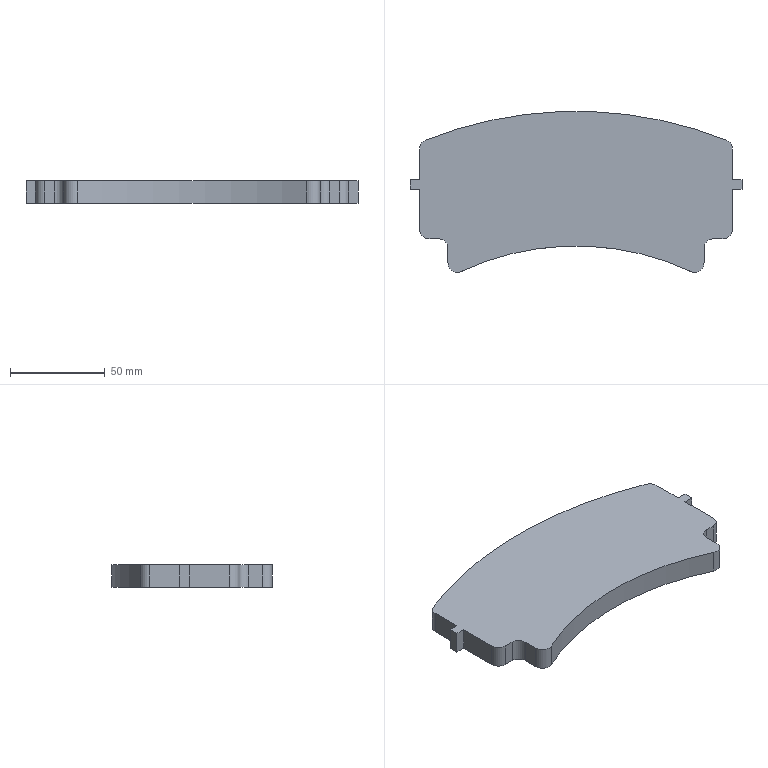Part | SolidWorks | features ICE 2, Extrusion 1, Fillet 1 | 1 solid | 26 faces | box 175 x 84.844 x 12 mm | volume 137582 mm3 | plane 16 | cylinder 10 | commonest cylinder face diameters 10 x8 286 x1 428 x1
STEP:
#1=CARTESIAN_POINT('',(-82.5,172.951,6.));
#2=VERTEX_POINT('',#1);
#3=CARTESIAN_POINT('',(-82.5,151.802,6.));
#4=VERTEX_POINT('',#3);
#5=CARTESIAN_POINT('',(-82.5,197.458,6.));
#6=DIRECTION('',(0.,-1.,0.));
#7=VECTOR('',#6,1000.);
#8=LINE('',#5,#7);
#9=EDGE_CURVE('',#2,#4,#8,.T.);
#10=ORIENTED_EDGE('',*,*,#9,.F.);
#11=CARTESIAN_POINT('',(-82.5,172.951,-6.));
#12=VERTEX_POINT('',#11);
#13=CARTESIAN_POINT('',(-82.5,172.951,-13.071));
#14=DIRECTION('',(0.,0.,1.));
#15=VECTOR('',#14,1000.);
#16=LINE('',#13,#15);
#17=EDGE_CURVE('',#12,#2,#16,.T.);
#18=ORIENTED_EDGE('',*,*,#17,.F.);
#19=CARTESIAN_POINT('',(-82.5,151.802,-6.));
#20=VERTEX_POINT('',#19);
#21=CARTESIAN_POINT('',(-82.5,197.458,-6.));
#22=DIRECTION('',(0.,-1.,0.));
#23=VECTOR('',#22,1000.);
#24=LINE('',#21,#23);
#25=EDGE_CURVE('',#12,#20,#24,.T.);
#26=ORIENTED_EDGE('',*,*,#25,.T.);
#27=CARTESIAN_POINT('',(-82.5,151.802,6.));
#28=DIRECTION('',(0.,0.,1.));
#29=VECTOR('',#28,1000.);
#30=LINE('',#27,#29);
#31=EDGE_CURVE('',#20,#4,#30,.T.);
#32=ORIENTED_EDGE('',*,*,#31,.T.);
#33=EDGE_LOOP('',(#10,#18,#26,#32));
#34=FACE_OUTER_BOUND('',#33,.T.);
#35=CARTESIAN_POINT('',(-82.5,197.458,6.));
#36=DIRECTION('',(1.,0.,0.));
#37=DIRECTION('',(0.,1.,0.));
#38=AXIS2_PLACEMENT_3D('',#35,#36,#37);
#39=PLANE('',#38);
#40=ADVANCED_FACE('',(#34),#39,.F.);
#41=CARTESIAN_POINT('',(82.5,177.951,6.));
#42=VERTEX_POINT('',#41);
#43=CARTESIAN_POINT('',(82.5,194.1,6.));
#44=VERTEX_POINT('',#43);
#45=CARTESIAN_POINT('',(82.5,197.458,6.));
#46=DIRECTION('',(0.,1.,0.));
#47=VECTOR('',#46,1000.);
#48=LINE('',#45,#47);
#49=EDGE_CURVE('',#42,#44,#48,.T.);
#50=ORIENTED_EDGE('',*,*,#49,.F.);
#51=CARTESIAN_POINT('',(82.5,177.951,-6.));
#52=VERTEX_POINT('',#51);
#53=CARTESIAN_POINT('',(82.5,177.951,-13.071));
#54=DIRECTION('',(0.,0.,1.));
#55=VECTOR('',#54,1000.);
#56=LINE('',#53,#55);
#57=EDGE_CURVE('',#52,#42,#56,.T.);
#58=ORIENTED_EDGE('',*,*,#57,.F.);
#59=CARTESIAN_POINT('',(82.5,194.1,-6.));
#60=VERTEX_POINT('',#59);
#61=CARTESIAN_POINT('',(82.5,197.458,-6.));
#62=DIRECTION('',(0.,1.,0.));
#63=VECTOR('',#62,1000.);
#64=LINE('',#61,#63);
#65=EDGE_CURVE('',#52,#60,#64,.T.);
#66=ORIENTED_EDGE('',*,*,#65,.T.);
#67=CARTESIAN_POINT('',(82.5,194.1,6.));
#68=DIRECTION('',(0.,0.,1.));
#69=VECTOR('',#68,1000.);
#70=LINE('',#67,#69);
#71=EDGE_CURVE('',#60,#44,#70,.T.);
#72=ORIENTED_EDGE('',*,*,#71,.T.);
#73=EDGE_LOOP('',(#50,#58,#66,#72));
#74=FACE_OUTER_BOUND('',#73,.T.);
#75=CARTESIAN_POINT('',(82.5,197.458,6.));
#76=DIRECTION('',(-1.,0.,0.));
#77=DIRECTION('',(0.,-1.,0.));
#78=AXIS2_PLACEMENT_3D('',#75,#76,#77);
#79=PLANE('',#78);
#80=ADVANCED_FACE('',(#74),#79,.F.);
#81=CARTESIAN_POINT('',(-60.389,129.623,-6.));
#82=VERTEX_POINT('',#81);
#83=CARTESIAN_POINT('',(60.389,129.623,-6.));
#84=VERTEX_POINT('',#83);
#85=CARTESIAN_POINT('',(0.,0.,-6.));
#86=DIRECTION('',(0.,0.,-1.));
#87=DIRECTION('',(1.,0.,0.));
#88=AXIS2_PLACEMENT_3D('',#85,#86,#87);
#89=CIRCLE('',#88,143.);
#90=EDGE_CURVE('',#82,#84,#89,.T.);
#91=ORIENTED_EDGE('',*,*,#90,.T.);
#92=CARTESIAN_POINT('',(60.389,129.623,6.));
#93=VERTEX_POINT('',#92);
#94=CARTESIAN_POINT('',(60.389,129.623,6.));
#95=DIRECTION('',(0.,0.,1.));
#96=VECTOR('',#95,1000.);
#97=LINE('',#94,#96);
#98=EDGE_CURVE('',#84,#93,#97,.T.);
#99=ORIENTED_EDGE('',*,*,#98,.T.);
#100=CARTESIAN_POINT('',(-60.389,129.623,6.));
#101=VERTEX_POINT('',#100);
#102=CARTESIAN_POINT('',(0.,0.,6.));
#103=DIRECTION('',(0.,0.,-1.));
#104=DIRECTION('',(1.,0.,0.));
#105=AXIS2_PLACEMENT_3D('',#102,#103,#104);
#106=CIRCLE('',#105,143.);
#107=EDGE_CURVE('',#101,#93,#106,.T.);
#108=ORIENTED_EDGE('',*,*,#107,.F.);
#109=CARTESIAN_POINT('',(-60.389,129.623,6.));
#110=DIRECTION('',(0.,0.,-1.));
#111=VECTOR('',#110,1000.);
#112=LINE('',#109,#111);
#113=EDGE_CURVE('',#101,#82,#112,.T.);
#114=ORIENTED_EDGE('',*,*,#113,.T.);
#115=EDGE_LOOP('',(#91,#99,#108,#114));
#116=FACE_OUTER_BOUND('',#115,.T.);
#117=CARTESIAN_POINT('',(0.,0.,6.));
#118=DIRECTION('',(0.,0.,-1.));
#119=DIRECTION('',(-1.,0.,0.));
#120=AXIS2_PLACEMENT_3D('',#117,#118,#119);
#121=CYLINDRICAL_SURFACE('',#120,143.);
#122=ADVANCED_FACE('',(#116),#121,.F.);
#123=CARTESIAN_POINT('',(82.5,151.802,-6.));
#124=VERTEX_POINT('',#123);
#125=CARTESIAN_POINT('',(82.5,172.951,-6.));
#126=VERTEX_POINT('',#125);
#127=CARTESIAN_POINT('',(82.5,197.458,-6.));
#128=DIRECTION('',(0.,1.,0.));
#129=VECTOR('',#128,1000.);
#130=LINE('',#127,#129);
#131=EDGE_CURVE('',#124,#126,#130,.T.);
#132=ORIENTED_EDGE('',*,*,#131,.T.);
#133=CARTESIAN_POINT('',(82.5,172.951,6.));
#134=VERTEX_POINT('',#133);
#135=CARTESIAN_POINT('',(82.5,172.951,-13.071));
#136=DIRECTION('',(0.,0.,1.));
#137=VECTOR('',#136,1000.);
#138=LINE('',#135,#137);
#139=EDGE_CURVE('',#126,#134,#138,.T.);
#140=ORIENTED_EDGE('',*,*,#139,.T.);
#141=CARTESIAN_POINT('',(82.5,151.802,6.));
#142=VERTEX_POINT('',#141);
#143=CARTESIAN_POINT('',(82.5,197.458,6.));
#144=DIRECTION('',(0.,1.,0.));
#145=VECTOR('',#144,1000.);
#146=LINE('',#143,#145);
#147=EDGE_CURVE('',#142,#134,#146,.T.);
#148=ORIENTED_EDGE('',*,*,#147,.F.);
#149=CARTESIAN_POINT('',(82.5,151.802,6.));
#150=DIRECTION('',(0.,0.,-1.));
#151=VECTOR('',#150,1000.);
#152=LINE('',#149,#151);
#153=EDGE_CURVE('',#142,#124,#152,.T.);
#154=ORIENTED_EDGE('',*,*,#153,.T.);
#155=EDGE_LOOP('',(#132,#140,#148,#154));
#156=FACE_OUTER_BOUND('',#155,.T.);
#157=CARTESIAN_POINT('',(82.5,197.458,6.));
#158=DIRECTION('',(-1.,0.,0.));
#159=DIRECTION('',(0.,-1.,0.));
#160=AXIS2_PLACEMENT_3D('',#157,#158,#159);
#161=PLANE('',#160);
#162=ADVANCED_FACE('',(#156),#161,.F.);
#163=CARTESIAN_POINT('',(79.354,198.743,6.));
#164=VERTEX_POINT('',#163);
#165=CARTESIAN_POINT('',(-79.354,198.743,6.));
#166=VERTEX_POINT('',#165);
#167=CARTESIAN_POINT('',(0.,0.,6.));
#168=DIRECTION('',(0.,0.,1.));
#169=DIRECTION('',(1.,0.,0.));
#170=AXIS2_PLACEMENT_3D('',#167,#168,#169);
#171=CIRCLE('',#170,214.);
#172=EDGE_CURVE('',#164,#166,#171,.T.);
#173=ORIENTED_EDGE('',*,*,#172,.F.);
#174=CARTESIAN_POINT('',(79.354,198.743,-6.));
#175=VERTEX_POINT('',#174);
#176=CARTESIAN_POINT('',(79.354,198.743,6.));
#177=DIRECTION('',(0.,0.,-1.));
#178=VECTOR('',#177,1000.);
#179=LINE('',#176,#178);
#180=EDGE_CURVE('',#164,#175,#179,.T.);
#181=ORIENTED_EDGE('',*,*,#180,.T.);
#182=CARTESIAN_POINT('',(-79.354,198.743,-6.));
#183=VERTEX_POINT('',#182);
#184=CARTESIAN_POINT('',(0.,0.,-6.));
#185=DIRECTION('',(0.,0.,1.));
#186=DIRECTION('',(1.,0.,0.));
#187=AXIS2_PLACEMENT_3D('',#184,#185,#186);
#188=CIRCLE('',#187,214.);
#189=EDGE_CURVE('',#175,#183,#188,.T.);
#190=ORIENTED_EDGE('',*,*,#189,.T.);
#191=CARTESIAN_POINT('',(-79.354,198.743,6.));
#192=DIRECTION('',(0.,0.,1.));
#193=VECTOR('',#192,1000.);
#194=LINE('',#191,#193);
#195=EDGE_CURVE('',#183,#166,#194,.T.);
#196=ORIENTED_EDGE('',*,*,#195,.T.);
#197=EDGE_LOOP('',(#173,#181,#190,#196));
#198=FACE_OUTER_BOUND('',#197,.T.);
#199=CARTESIAN_POINT('',(0.,0.,6.));
#200=DIRECTION('',(0.,0.,-1.));
#201=DIRECTION('',(-1.,0.,0.));
#202=AXIS2_PLACEMENT_3D('',#199,#200,#201);
#203=CYLINDRICAL_SURFACE('',#202,214.);
#204=ADVANCED_FACE('',(#198),#203,.T.);
#205=CARTESIAN_POINT('',(-82.5,194.1,-6.));
#206=VERTEX_POINT('',#205);
#207=CARTESIAN_POINT('',(-82.5,177.951,-6.));
#208=VERTEX_POINT('',#207);
#209=CARTESIAN_POINT('',(-82.5,197.458,-6.));
#210=DIRECTION('',(0.,-1.,0.));
#211=VECTOR('',#210,1000.);
#212=LINE('',#209,#211);
#213=EDGE_CURVE('',#206,#208,#212,.T.);
#214=ORIENTED_EDGE('',*,*,#213,.T.);
#215=CARTESIAN_POINT('',(-82.5,177.951,6.));
#216=VERTEX_POINT('',#215);
#217=CARTESIAN_POINT('',(-82.5,177.951,-13.071));
#218=DIRECTION('',(0.,0.,1.));
#219=VECTOR('',#218,1000.);
#220=LINE('',#217,#219);
#221=EDGE_CURVE('',#208,#216,#220,.T.);
#222=ORIENTED_EDGE('',*,*,#221,.T.);
#223=CARTESIAN_POINT('',(-82.5,194.1,6.));
#224=VERTEX_POINT('',#223);
#225=CARTESIAN_POINT('',(-82.5,197.458,6.));
#226=DIRECTION('',(0.,-1.,0.));
#227=VECTOR('',#226,1000.);
#228=LINE('',#225,#227);
#229=EDGE_CURVE('',#224,#216,#228,.T.);
#230=ORIENTED_EDGE('',*,*,#229,.F.);
#231=CARTESIAN_POINT('',(-82.5,194.1,6.));
#232=DIRECTION('',(0.,0.,-1.));
#233=VECTOR('',#232,1000.);
#234=LINE('',#231,#233);
#235=EDGE_CURVE('',#224,#206,#234,.T.);
#236=ORIENTED_EDGE('',*,*,#235,.T.);
#237=EDGE_LOOP('',(#214,#222,#230,#236));
#238=FACE_OUTER_BOUND('',#237,.T.);
#239=CARTESIAN_POINT('',(-82.5,197.458,6.));
#240=DIRECTION('',(1.,0.,0.));
#241=DIRECTION('',(0.,1.,0.));
#242=AXIS2_PLACEMENT_3D('',#239,#240,#241);
#243=PLANE('',#242);
#244=ADVANCED_FACE('',(#238),#243,.F.);
#245=ORIENTED_EDGE('',*,*,#147,.T.);
#246=CARTESIAN_POINT('',(87.5,172.951,6.));
#247=VERTEX_POINT('',#246);
#248=CARTESIAN_POINT('',(82.5,172.951,6.));
#249=DIRECTION('',(1.,0.,0.));
#250=VECTOR('',#249,1000.);
#251=LINE('',#248,#250);
#252=EDGE_CURVE('',#134,#247,#251,.T.);
#253=ORIENTED_EDGE('',*,*,#252,.T.);
#254=CARTESIAN_POINT('',(87.5,177.951,6.));
#255=VERTEX_POINT('',#254);
#256=CARTESIAN_POINT('',(87.5,172.951,6.));
#257=DIRECTION('',(0.,1.,0.));
#258=VECTOR('',#257,1000.);
#259=LINE('',#256,#258);
#260=EDGE_CURVE('',#247,#255,#259,.T.);
#261=ORIENTED_EDGE('',*,*,#260,.T.);
#262=CARTESIAN_POINT('',(82.5,177.951,6.));
#263=DIRECTION('',(-1.,0.,0.));
#264=VECTOR('',#263,1000.);
#265=LINE('',#262,#264);
#266=EDGE_CURVE('',#255,#42,#265,.T.);
#267=ORIENTED_EDGE('',*,*,#266,.T.);
#268=ORIENTED_EDGE('',*,*,#49,.T.);
#269=CARTESIAN_POINT('',(77.5,194.1,6.));
#270=DIRECTION('',(0.,0.,1.));
#271=DIRECTION('',(1.,0.,0.));
#272=AXIS2_PLACEMENT_3D('',#269,#270,#271);
#273=CIRCLE('',#272,5.);
#274=EDGE_CURVE('',#44,#164,#273,.T.);
#275=ORIENTED_EDGE('',*,*,#274,.T.);
#276=ORIENTED_EDGE('',*,*,#172,.T.);
#277=CARTESIAN_POINT('',(-77.5,194.1,6.));
#278=DIRECTION('',(0.,0.,1.));
#279=DIRECTION('',(1.,0.,0.));
#280=AXIS2_PLACEMENT_3D('',#277,#278,#279);
#281=CIRCLE('',#280,5.);
#282=EDGE_CURVE('',#166,#224,#281,.T.);
#283=ORIENTED_EDGE('',*,*,#282,.T.);
#284=ORIENTED_EDGE('',*,*,#229,.T.);
#285=CARTESIAN_POINT('',(-87.5,177.951,6.));
#286=VERTEX_POINT('',#285);
#287=CARTESIAN_POINT('',(-82.5,177.951,6.));
#288=DIRECTION('',(-1.,0.,0.));
#289=VECTOR('',#288,1000.);
#290=LINE('',#287,#289);
#291=EDGE_CURVE('',#216,#286,#290,.T.);
#292=ORIENTED_EDGE('',*,*,#291,.T.);
#293=CARTESIAN_POINT('',(-87.5,172.951,6.));
#294=VERTEX_POINT('',#293);
#295=CARTESIAN_POINT('',(-87.5,172.951,6.));
#296=DIRECTION('',(0.,-1.,0.));
#297=VECTOR('',#296,1000.);
#298=LINE('',#295,#297);
#299=EDGE_CURVE('',#286,#294,#298,.T.);
#300=ORIENTED_EDGE('',*,*,#299,.T.);
#301=CARTESIAN_POINT('',(-82.5,172.951,6.));
#302=DIRECTION('',(1.,0.,0.));
#303=VECTOR('',#302,1000.);
#304=LINE('',#301,#303);
#305=EDGE_CURVE('',#294,#2,#304,.T.);
#306=ORIENTED_EDGE('',*,*,#305,.T.);
#307=ORIENTED_EDGE('',*,*,#9,.T.);
#308=CARTESIAN_POINT('',(-77.5,146.802,6.));
#309=VERTEX_POINT('',#308);
#310=CARTESIAN_POINT('',(-77.5,151.802,6.));
#311=DIRECTION('',(0.,0.,1.));
#312=DIRECTION('',(1.,0.,0.));
#313=AXIS2_PLACEMENT_3D('',#310,#311,#312);
#314=CIRCLE('',#313,5.);
#315=EDGE_CURVE('',#4,#309,#314,.T.);
#316=ORIENTED_EDGE('',*,*,#315,.T.);
#317=CARTESIAN_POINT('',(-72.5,146.802,6.));
#318=VERTEX_POINT('',#317);
#319=CARTESIAN_POINT('',(-82.5,146.802,6.));
#320=DIRECTION('',(-1.,0.,0.));
#321=VECTOR('',#320,1000.);
#322=LINE('',#319,#321);
#323=EDGE_CURVE('',#318,#309,#322,.T.);
#324=ORIENTED_EDGE('',*,*,#323,.F.);
#325=CARTESIAN_POINT('',(-67.5,141.802,6.));
#326=VERTEX_POINT('',#325);
#327=CARTESIAN_POINT('',(-72.5,141.802,6.));
#328=DIRECTION('',(0.,0.,-1.));
#329=DIRECTION('',(1.,0.,0.));
#330=AXIS2_PLACEMENT_3D('',#327,#328,#329);
#331=CIRCLE('',#330,5.);
#332=EDGE_CURVE('',#318,#326,#331,.T.);
#333=ORIENTED_EDGE('',*,*,#332,.T.);
#334=CARTESIAN_POINT('',(-67.5,134.156,6.));
#335=VERTEX_POINT('',#334);
#336=CARTESIAN_POINT('',(-67.5,116.802,6.));
#337=DIRECTION('',(0.,1.,0.));
#338=VECTOR('',#337,1000.);
#339=LINE('',#336,#338);
#340=EDGE_CURVE('',#335,#326,#339,.T.);
#341=ORIENTED_EDGE('',*,*,#340,.F.);
#342=CARTESIAN_POINT('',(-62.5,134.156,6.));
#343=DIRECTION('',(0.,0.,1.));
#344=DIRECTION('',(1.,0.,0.));
#345=AXIS2_PLACEMENT_3D('',#342,#343,#344);
#346=CIRCLE('',#345,5.);
#347=EDGE_CURVE('',#335,#101,#346,.T.);
#348=ORIENTED_EDGE('',*,*,#347,.T.);
#349=ORIENTED_EDGE('',*,*,#107,.T.);
#350=CARTESIAN_POINT('',(67.5,134.156,6.));
#351=VERTEX_POINT('',#350);
#352=CARTESIAN_POINT('',(62.5,134.156,6.));
#353=DIRECTION('',(0.,0.,1.));
#354=DIRECTION('',(1.,0.,0.));
#355=AXIS2_PLACEMENT_3D('',#352,#353,#354);
#356=CIRCLE('',#355,5.);
#357=EDGE_CURVE('',#93,#351,#356,.T.);
#358=ORIENTED_EDGE('',*,*,#357,.T.);
#359=CARTESIAN_POINT('',(67.5,141.802,6.));
#360=VERTEX_POINT('',#359);
#361=CARTESIAN_POINT('',(67.5,116.802,6.));
#362=DIRECTION('',(0.,-1.,0.));
#363=VECTOR('',#362,1000.);
#364=LINE('',#361,#363);
#365=EDGE_CURVE('',#360,#351,#364,.T.);
#366=ORIENTED_EDGE('',*,*,#365,.F.);
#367=CARTESIAN_POINT('',(72.5,146.802,6.));
#368=VERTEX_POINT('',#367);
#369=CARTESIAN_POINT('',(72.5,141.802,6.));
#370=DIRECTION('',(0.,0.,-1.));
#371=DIRECTION('',(1.,0.,0.));
#372=AXIS2_PLACEMENT_3D('',#369,#370,#371);
#373=CIRCLE('',#372,5.);
#374=EDGE_CURVE('',#360,#368,#373,.T.);
#375=ORIENTED_EDGE('',*,*,#374,.T.);
#376=CARTESIAN_POINT('',(77.5,146.802,6.));
#377=VERTEX_POINT('',#376);
#378=CARTESIAN_POINT('',(82.5,146.802,6.));
#379=DIRECTION('',(-1.,0.,0.));
#380=VECTOR('',#379,1000.);
#381=LINE('',#378,#380);
#382=EDGE_CURVE('',#377,#368,#381,.T.);
#383=ORIENTED_EDGE('',*,*,#382,.F.);
#384=CARTESIAN_POINT('',(77.5,151.802,6.));
#385=DIRECTION('',(0.,0.,1.));
#386=DIRECTION('',(1.,0.,0.));
#387=AXIS2_PLACEMENT_3D('',#384,#385,#386);
#388=CIRCLE('',#387,5.);
#389=EDGE_CURVE('',#377,#142,#388,.T.);
#390=ORIENTED_EDGE('',*,*,#389,.T.);
#391=EDGE_LOOP('',(#245,#253,#261,#267,#268,#275,#276,#283,#284,#292,#300,#306,#307,#316,#324,#333,#341,#348,#349,#358,#366,#375,#383,#390));
#392=FACE_OUTER_BOUND('',#391,.T.);
#393=CARTESIAN_POINT('',(0.,0.,6.));
#394=DIRECTION('',(0.,0.,1.));
#395=DIRECTION('',(1.,0.,0.));
#396=AXIS2_PLACEMENT_3D('',#393,#394,#395);
#397=PLANE('',#396);
#398=ADVANCED_FACE('',(#392),#397,.T.);
#399=ORIENTED_EDGE('',*,*,#189,.F.);
#400=CARTESIAN_POINT('',(77.5,194.1,-6.));
#401=DIRECTION('',(0.,0.,-1.));
#402=DIRECTION('',(1.,0.,0.));
#403=AXIS2_PLACEMENT_3D('',#400,#401,#402);
#404=CIRCLE('',#403,5.);
#405=EDGE_CURVE('',#175,#60,#404,.T.);
#406=ORIENTED_EDGE('',*,*,#405,.T.);
#407=ORIENTED_EDGE('',*,*,#65,.F.);
#408=CARTESIAN_POINT('',(87.5,177.951,-6.));
#409=VERTEX_POINT('',#408);
#410=CARTESIAN_POINT('',(82.5,177.951,-6.));
#411=DIRECTION('',(1.,0.,0.));
#412=VECTOR('',#411,1000.);
#413=LINE('',#410,#412);
#414=EDGE_CURVE('',#52,#409,#413,.T.);
#415=ORIENTED_EDGE('',*,*,#414,.T.);
#416=CARTESIAN_POINT('',(87.5,172.951,-6.));
#417=VERTEX_POINT('',#416);
#418=CARTESIAN_POINT('',(87.5,172.951,-6.));
#419=DIRECTION('',(0.,-1.,0.));
#420=VECTOR('',#419,1000.);
#421=LINE('',#418,#420);
#422=EDGE_CURVE('',#409,#417,#421,.T.);
#423=ORIENTED_EDGE('',*,*,#422,.T.);
#424=CARTESIAN_POINT('',(82.5,172.951,-6.));
#425=DIRECTION('',(-1.,0.,0.));
#426=VECTOR('',#425,1000.);
#427=LINE('',#424,#426);
#428=EDGE_CURVE('',#417,#126,#427,.T.);
#429=ORIENTED_EDGE('',*,*,#428,.T.);
#430=ORIENTED_EDGE('',*,*,#131,.F.);
#431=CARTESIAN_POINT('',(77.5,146.802,-6.));
#432=VERTEX_POINT('',#431);
#433=CARTESIAN_POINT('',(77.5,151.802,-6.));
#434=DIRECTION('',(0.,0.,-1.));
#435=DIRECTION('',(1.,0.,0.));
#436=AXIS2_PLACEMENT_3D('',#433,#434,#435);
#437=CIRCLE('',#436,5.);
#438=EDGE_CURVE('',#124,#432,#437,.T.);
#439=ORIENTED_EDGE('',*,*,#438,.T.);
#440=CARTESIAN_POINT('',(72.5,146.802,-6.));
#441=VERTEX_POINT('',#440);
#442=CARTESIAN_POINT('',(0.,146.802,-6.));
#443=DIRECTION('',(-1.,0.,0.));
#444=VECTOR('',#443,1000.);
#445=LINE('',#442,#444);
#446=EDGE_CURVE('',#432,#441,#445,.T.);
#447=ORIENTED_EDGE('',*,*,#446,.T.);
#448=CARTESIAN_POINT('',(67.5,141.802,-6.));
#449=VERTEX_POINT('',#448);
#450=CARTESIAN_POINT('',(72.5,141.802,-6.));
#451=DIRECTION('',(0.,0.,1.));
#452=DIRECTION('',(1.,0.,0.));
#453=AXIS2_PLACEMENT_3D('',#450,#451,#452);
#454=CIRCLE('',#453,5.);
#455=EDGE_CURVE('',#441,#449,#454,.T.);
#456=ORIENTED_EDGE('',*,*,#455,.T.);
#457=CARTESIAN_POINT('',(67.5,134.156,-6.));
#458=VERTEX_POINT('',#457);
#459=CARTESIAN_POINT('',(67.5,0.,-6.));
#460=DIRECTION('',(0.,-1.,0.));
#461=VECTOR('',#460,1000.);
#462=LINE('',#459,#461);
#463=EDGE_CURVE('',#449,#458,#462,.T.);
#464=ORIENTED_EDGE('',*,*,#463,.T.);
#465=CARTESIAN_POINT('',(62.5,134.156,-6.));
#466=DIRECTION('',(0.,0.,-1.));
#467=DIRECTION('',(1.,0.,0.));
#468=AXIS2_PLACEMENT_3D('',#465,#466,#467);
#469=CIRCLE('',#468,5.);
#470=EDGE_CURVE('',#458,#84,#469,.T.);
#471=ORIENTED_EDGE('',*,*,#470,.T.);
#472=ORIENTED_EDGE('',*,*,#90,.F.);
#473=CARTESIAN_POINT('',(-67.5,134.156,-6.));
#474=VERTEX_POINT('',#473);
#475=CARTESIAN_POINT('',(-62.5,134.156,-6.));
#476=DIRECTION('',(0.,0.,-1.));
#477=DIRECTION('',(1.,0.,0.));
#478=AXIS2_PLACEMENT_3D('',#475,#476,#477);
#479=CIRCLE('',#478,5.);
#480=EDGE_CURVE('',#82,#474,#479,.T.);
#481=ORIENTED_EDGE('',*,*,#480,.T.);
#482=CARTESIAN_POINT('',(-67.5,141.802,-6.));
#483=VERTEX_POINT('',#482);
#484=CARTESIAN_POINT('',(-67.5,0.,-6.));
#485=DIRECTION('',(0.,1.,0.));
#486=VECTOR('',#485,1000.);
#487=LINE('',#484,#486);
#488=EDGE_CURVE('',#474,#483,#487,.T.);
#489=ORIENTED_EDGE('',*,*,#488,.T.);
#490=CARTESIAN_POINT('',(-72.5,146.802,-6.));
#491=VERTEX_POINT('',#490);
#492=CARTESIAN_POINT('',(-72.5,141.802,-6.));
#493=DIRECTION('',(0.,0.,1.));
#494=DIRECTION('',(1.,0.,0.));
#495=AXIS2_PLACEMENT_3D('',#492,#493,#494);
#496=CIRCLE('',#495,5.);
#497=EDGE_CURVE('',#483,#491,#496,.T.);
#498=ORIENTED_EDGE('',*,*,#497,.T.);
#499=CARTESIAN_POINT('',(-77.5,146.802,-6.));
#500=VERTEX_POINT('',#499);
#501=CARTESIAN_POINT('',(0.,146.802,-6.));
#502=DIRECTION('',(-1.,0.,0.));
#503=VECTOR('',#502,1000.);
#504=LINE('',#501,#503);
#505=EDGE_CURVE('',#491,#500,#504,.T.);
#506=ORIENTED_EDGE('',*,*,#505,.T.);
#507=CARTESIAN_POINT('',(-77.5,151.802,-6.));
#508=DIRECTION('',(0.,0.,-1.));
#509=DIRECTION('',(1.,0.,0.));
#510=AXIS2_PLACEMENT_3D('',#507,#508,#509);
#511=CIRCLE('',#510,5.);
#512=EDGE_CURVE('',#500,#20,#511,.T.);
#513=ORIENTED_EDGE('',*,*,#512,.T.);
#514=ORIENTED_EDGE('',*,*,#25,.F.);
#515=CARTESIAN_POINT('',(-87.5,172.951,-6.));
#516=VERTEX_POINT('',#515);
#517=CARTESIAN_POINT('',(-82.5,172.951,-6.));
#518=DIRECTION('',(-1.,0.,0.));
#519=VECTOR('',#518,1000.);
#520=LINE('',#517,#519);
#521=EDGE_CURVE('',#12,#516,#520,.T.);
#522=ORIENTED_EDGE('',*,*,#521,.T.);
#523=CARTESIAN_POINT('',(-87.5,177.951,-6.));
#524=VERTEX_POINT('',#523);
#525=CARTESIAN_POINT('',(-87.5,172.951,-6.));
#526=DIRECTION('',(0.,1.,0.));
#527=VECTOR('',#526,1000.);
#528=LINE('',#525,#527);
#529=EDGE_CURVE('',#516,#524,#528,.T.);
#530=ORIENTED_EDGE('',*,*,#529,.T.);
#531=CARTESIAN_POINT('',(-82.5,177.951,-6.));
#532=DIRECTION('',(1.,0.,0.));
#533=VECTOR('',#532,1000.);
#534=LINE('',#531,#533);
#535=EDGE_CURVE('',#524,#208,#534,.T.);
#536=ORIENTED_EDGE('',*,*,#535,.T.);
#537=ORIENTED_EDGE('',*,*,#213,.F.);
#538=CARTESIAN_POINT('',(-77.5,194.1,-6.));
#539=DIRECTION('',(0.,0.,-1.));
#540=DIRECTION('',(1.,0.,0.));
#541=AXIS2_PLACEMENT_3D('',#538,#539,#540);
#542=CIRCLE('',#541,5.);
#543=EDGE_CURVE('',#206,#183,#542,.T.);
#544=ORIENTED_EDGE('',*,*,#543,.T.);
#545=EDGE_LOOP('',(#399,#406,#407,#415,#423,#429,#430,#439,#447,#456,#464,#471,#472,#481,#489,#498,#506,#513,#514,#522,#530,#536,#537,#544));
#546=FACE_OUTER_BOUND('',#545,.T.);
#547=CARTESIAN_POINT('',(0.,0.,-6.));
#548=DIRECTION('',(0.,0.,1.));
#549=DIRECTION('',(1.,0.,0.));
#550=AXIS2_PLACEMENT_3D('',#547,#548,#549);
#551=PLANE('',#550);
#552=ADVANCED_FACE('',(#546),#551,.F.);
#553=ORIENTED_EDGE('',*,*,#463,.F.);
#554=CARTESIAN_POINT('',(67.5,141.802,6.));
#555=DIRECTION('',(0.,0.,1.));
#556=VECTOR('',#555,1000.);
#557=LINE('',#554,#556);
#558=EDGE_CURVE('',#449,#360,#557,.T.);
#559=ORIENTED_EDGE('',*,*,#558,.T.);
#560=ORIENTED_EDGE('',*,*,#365,.T.);
#561=CARTESIAN_POINT('',(67.5,134.156,-24.));
#562=DIRECTION('',(0.,0.,-1.));
#563=VECTOR('',#562,1000.);
#564=LINE('',#561,#563);
#565=EDGE_CURVE('',#351,#458,#564,.T.);
#566=ORIENTED_EDGE('',*,*,#565,.T.);
#567=EDGE_LOOP('',(#553,#559,#560,#566));
#568=FACE_OUTER_BOUND('',#567,.T.);
#569=CARTESIAN_POINT('',(67.5,116.802,-24.));
#570=DIRECTION('',(-1.,0.,0.));
#571=DIRECTION('',(0.,0.,1.));
#572=AXIS2_PLACEMENT_3D('',#569,#570,#571);
#573=PLANE('',#572);
#574=ADVANCED_FACE('',(#568),#573,.F.);
#575=ORIENTED_EDGE('',*,*,#446,.F.);
#576=CARTESIAN_POINT('',(77.5,146.802,-24.));
#577=DIRECTION('',(0.,0.,1.));
#578=VECTOR('',#577,1000.);
#579=LINE('',#576,#578);
#580=EDGE_CURVE('',#432,#377,#579,.T.);
#581=ORIENTED_EDGE('',*,*,#580,.T.);
#582=ORIENTED_EDGE('',*,*,#382,.T.);
#583=CARTESIAN_POINT('',(72.5,146.802,-6.));
#584=DIRECTION('',(0.,0.,-1.));
#585=VECTOR('',#584,1000.);
#586=LINE('',#583,#585);
#587=EDGE_CURVE('',#368,#441,#586,.T.);
#588=ORIENTED_EDGE('',*,*,#587,.T.);
#589=EDGE_LOOP('',(#575,#581,#582,#588));
#590=FACE_OUTER_BOUND('',#589,.T.);
#591=CARTESIAN_POINT('',(82.5,146.802,-24.));
#592=DIRECTION('',(0.,1.,0.));
#593=DIRECTION('',(0.,0.,1.));
#594=AXIS2_PLACEMENT_3D('',#591,#592,#593);
#595=PLANE('',#594);
#596=ADVANCED_FACE('',(#590),#595,.F.);
#597=ORIENTED_EDGE('',*,*,#505,.F.);
#598=CARTESIAN_POINT('',(-72.5,146.802,6.));
#599=DIRECTION('',(0.,0.,1.));
#600=VECTOR('',#599,1000.);
#601=LINE('',#598,#600);
#602=EDGE_CURVE('',#491,#318,#601,.T.);
#603=ORIENTED_EDGE('',*,*,#602,.T.);
#604=ORIENTED_EDGE('',*,*,#323,.T.);
#605=CARTESIAN_POINT('',(-77.5,146.802,-24.));
#606=DIRECTION('',(0.,0.,-1.));
#607=VECTOR('',#606,1000.);
#608=LINE('',#605,#607);
#609=EDGE_CURVE('',#309,#500,#608,.T.);
#610=ORIENTED_EDGE('',*,*,#609,.T.);
#611=EDGE_LOOP('',(#597,#603,#604,#610));
#612=FACE_OUTER_BOUND('',#611,.T.);
#613=CARTESIAN_POINT('',(-82.5,146.802,-24.));
#614=DIRECTION('',(0.,1.,0.));
#615=DIRECTION('',(0.,0.,1.));
#616=AXIS2_PLACEMENT_3D('',#613,#614,#615);
#617=PLANE('',#616);
#618=ADVANCED_FACE('',(#612),#617,.F.);
#619=ORIENTED_EDGE('',*,*,#488,.F.);
#620=CARTESIAN_POINT('',(-67.5,134.156,-24.));
#621=DIRECTION('',(0.,0.,1.));
#622=VECTOR('',#621,1000.);
#623=LINE('',#620,#622);
#624=EDGE_CURVE('',#474,#335,#623,.T.);
#625=ORIENTED_EDGE('',*,*,#624,.T.);
#626=ORIENTED_EDGE('',*,*,#340,.T.);
#627=CARTESIAN_POINT('',(-67.5,141.802,-6.));
#628=DIRECTION('',(0.,0.,-1.));
#629=VECTOR('',#628,1000.);
#630=LINE('',#627,#629);
#631=EDGE_CURVE('',#326,#483,#630,.T.);
#632=ORIENTED_EDGE('',*,*,#631,.T.);
#633=EDGE_LOOP('',(#619,#625,#626,#632));
#634=FACE_OUTER_BOUND('',#633,.T.);
#635=CARTESIAN_POINT('',(-67.5,116.802,-24.));
#636=DIRECTION('',(1.,0.,0.));
#637=DIRECTION('',(0.,0.,-1.));
#638=AXIS2_PLACEMENT_3D('',#635,#636,#637);
#639=PLANE('',#638);
#640=ADVANCED_FACE('',(#634),#639,.F.);
#641=ORIENTED_EDGE('',*,*,#274,.F.);
#642=ORIENTED_EDGE('',*,*,#71,.F.);
#643=ORIENTED_EDGE('',*,*,#405,.F.);
#644=ORIENTED_EDGE('',*,*,#180,.F.);
#645=EDGE_LOOP('',(#641,#642,#643,#644));
#646=FACE_OUTER_BOUND('',#645,.T.);
#647=CARTESIAN_POINT('',(77.5,194.1,6.));
#648=DIRECTION('',(0.,0.,-1.));
#649=DIRECTION('',(-1.,0.,0.));
#650=AXIS2_PLACEMENT_3D('',#647,#648,#649);
#651=CYLINDRICAL_SURFACE('',#650,5.);
#652=ADVANCED_FACE('',(#646),#651,.T.);
#653=ORIENTED_EDGE('',*,*,#438,.F.);
#654=ORIENTED_EDGE('',*,*,#153,.F.);
#655=ORIENTED_EDGE('',*,*,#389,.F.);
#656=ORIENTED_EDGE('',*,*,#580,.F.);
#657=EDGE_LOOP('',(#653,#654,#655,#656));
#658=FACE_OUTER_BOUND('',#657,.T.);
#659=CARTESIAN_POINT('',(77.5,151.802,-24.));
#660=DIRECTION('',(0.,0.,1.));
#661=DIRECTION('',(1.,0.,0.));
#662=AXIS2_PLACEMENT_3D('',#659,#660,#661);
#663=CYLINDRICAL_SURFACE('',#662,5.);
#664=ADVANCED_FACE('',(#658),#663,.T.);
#665=ORIENTED_EDGE('',*,*,#455,.F.);
#666=ORIENTED_EDGE('',*,*,#587,.F.);
#667=ORIENTED_EDGE('',*,*,#374,.F.);
#668=ORIENTED_EDGE('',*,*,#558,.F.);
#669=EDGE_LOOP('',(#665,#666,#667,#668));
#670=FACE_OUTER_BOUND('',#669,.T.);
#671=CARTESIAN_POINT('',(72.5,141.802,-24.));
#672=DIRECTION('',(0.,0.,-1.));
#673=DIRECTION('',(-1.,0.,0.));
#674=AXIS2_PLACEMENT_3D('',#671,#672,#673);
#675=CYLINDRICAL_SURFACE('',#674,5.);
#676=ADVANCED_FACE('',(#670),#675,.F.);
#677=ORIENTED_EDGE('',*,*,#470,.F.);
#678=ORIENTED_EDGE('',*,*,#565,.F.);
#679=ORIENTED_EDGE('',*,*,#357,.F.);
#680=ORIENTED_EDGE('',*,*,#98,.F.);
#681=EDGE_LOOP('',(#677,#678,#679,#680));
#682=FACE_OUTER_BOUND('',#681,.T.);
#683=CARTESIAN_POINT('',(62.5,134.156,6.));
#684=DIRECTION('',(0.,0.,-1.));
#685=DIRECTION('',(-1.,0.,0.));
#686=AXIS2_PLACEMENT_3D('',#683,#684,#685);
#687=CYLINDRICAL_SURFACE('',#686,5.);
#688=ADVANCED_FACE('',(#682),#687,.T.);
#689=ORIENTED_EDGE('',*,*,#347,.F.);
#690=ORIENTED_EDGE('',*,*,#624,.F.);
#691=ORIENTED_EDGE('',*,*,#480,.F.);
#692=ORIENTED_EDGE('',*,*,#113,.F.);
#693=EDGE_LOOP('',(#689,#690,#691,#692));
#694=FACE_OUTER_BOUND('',#693,.T.);
#695=CARTESIAN_POINT('',(-62.5,134.156,6.));
#696=DIRECTION('',(0.,0.,-1.));
#697=DIRECTION('',(-1.,0.,0.));
#698=AXIS2_PLACEMENT_3D('',#695,#696,#697);
#699=CYLINDRICAL_SURFACE('',#698,5.);
#700=ADVANCED_FACE('',(#694),#699,.T.);
#701=ORIENTED_EDGE('',*,*,#497,.F.);
#702=ORIENTED_EDGE('',*,*,#631,.F.);
#703=ORIENTED_EDGE('',*,*,#332,.F.);
#704=ORIENTED_EDGE('',*,*,#602,.F.);
#705=EDGE_LOOP('',(#701,#702,#703,#704));
#706=FACE_OUTER_BOUND('',#705,.T.);
#707=CARTESIAN_POINT('',(-72.5,141.802,-24.));
#708=DIRECTION('',(0.,0.,-1.));
#709=DIRECTION('',(-1.,0.,0.));
#710=AXIS2_PLACEMENT_3D('',#707,#708,#709);
#711=CYLINDRICAL_SURFACE('',#710,5.);
#712=ADVANCED_FACE('',(#706),#711,.F.);
#713=ORIENTED_EDGE('',*,*,#512,.F.);
#714=ORIENTED_EDGE('',*,*,#609,.F.);
#715=ORIENTED_EDGE('',*,*,#315,.F.);
#716=ORIENTED_EDGE('',*,*,#31,.F.);
#717=EDGE_LOOP('',(#713,#714,#715,#716));
#718=FACE_OUTER_BOUND('',#717,.T.);
#719=CARTESIAN_POINT('',(-77.5,151.802,6.));
#720=DIRECTION('',(0.,0.,1.));
#721=DIRECTION('',(1.,0.,0.));
#722=AXIS2_PLACEMENT_3D('',#719,#720,#721);
#723=CYLINDRICAL_SURFACE('',#722,5.);
#724=ADVANCED_FACE('',(#718),#723,.T.);
#725=ORIENTED_EDGE('',*,*,#282,.F.);
#726=ORIENTED_EDGE('',*,*,#195,.F.);
#727=ORIENTED_EDGE('',*,*,#543,.F.);
#728=ORIENTED_EDGE('',*,*,#235,.F.);
#729=EDGE_LOOP('',(#725,#726,#727,#728));
#730=FACE_OUTER_BOUND('',#729,.T.);
#731=CARTESIAN_POINT('',(-77.5,194.1,6.));
#732=DIRECTION('',(0.,0.,-1.));
#733=DIRECTION('',(-1.,0.,0.));
#734=AXIS2_PLACEMENT_3D('',#731,#732,#733);
#735=CYLINDRICAL_SURFACE('',#734,5.);
#736=ADVANCED_FACE('',(#730),#735,.T.);
#737=ORIENTED_EDGE('',*,*,#414,.F.);
#738=ORIENTED_EDGE('',*,*,#57,.T.);
#739=ORIENTED_EDGE('',*,*,#266,.F.);
#740=CARTESIAN_POINT('',(87.5,177.951,-13.071));
#741=DIRECTION('',(0.,0.,1.));
#742=VECTOR('',#741,1000.);
#743=LINE('',#740,#742);
#744=EDGE_CURVE('',#409,#255,#743,.T.);
#745=ORIENTED_EDGE('',*,*,#744,.F.);
#746=EDGE_LOOP('',(#737,#738,#739,#745));
#747=FACE_OUTER_BOUND('',#746,.T.);
#748=CARTESIAN_POINT('',(82.5,177.951,-13.071));
#749=DIRECTION('',(0.,1.,0.));
#750=DIRECTION('',(-1.,0.,0.));
#751=AXIS2_PLACEMENT_3D('',#748,#749,#750);
#752=PLANE('',#751);
#753=ADVANCED_FACE('',(#747),#752,.T.);
#754=ORIENTED_EDGE('',*,*,#422,.F.);
#755=ORIENTED_EDGE('',*,*,#744,.T.);
#756=ORIENTED_EDGE('',*,*,#260,.F.);
#757=CARTESIAN_POINT('',(87.5,172.951,-13.071));
#758=DIRECTION('',(0.,0.,1.));
#759=VECTOR('',#758,1000.);
#760=LINE('',#757,#759);
#761=EDGE_CURVE('',#417,#247,#760,.T.);
#762=ORIENTED_EDGE('',*,*,#761,.F.);
#763=EDGE_LOOP('',(#754,#755,#756,#762));
#764=FACE_OUTER_BOUND('',#763,.T.);
#765=CARTESIAN_POINT('',(87.5,172.951,-13.071));
#766=DIRECTION('',(1.,0.,0.));
#767=DIRECTION('',(0.,0.,-1.));
#768=AXIS2_PLACEMENT_3D('',#765,#766,#767);
#769=PLANE('',#768);
#770=ADVANCED_FACE('',(#764),#769,.T.);
#771=ORIENTED_EDGE('',*,*,#428,.F.);
#772=ORIENTED_EDGE('',*,*,#761,.T.);
#773=ORIENTED_EDGE('',*,*,#252,.F.);
#774=ORIENTED_EDGE('',*,*,#139,.F.);
#775=EDGE_LOOP('',(#771,#772,#773,#774));
#776=FACE_OUTER_BOUND('',#775,.T.);
#777=CARTESIAN_POINT('',(82.5,172.951,-13.071));
#778=DIRECTION('',(0.,-1.,0.));
#779=DIRECTION('',(0.,0.,-1.));
#780=AXIS2_PLACEMENT_3D('',#777,#778,#779);
#781=PLANE('',#780);
#782=ADVANCED_FACE('',(#776),#781,.T.);
#783=ORIENTED_EDGE('',*,*,#521,.F.);
#784=ORIENTED_EDGE('',*,*,#17,.T.);
#785=ORIENTED_EDGE('',*,*,#305,.F.);
#786=CARTESIAN_POINT('',(-87.5,172.951,-13.071));
#787=DIRECTION('',(0.,0.,1.));
#788=VECTOR('',#787,1000.);
#789=LINE('',#786,#788);
#790=EDGE_CURVE('',#516,#294,#789,.T.);
#791=ORIENTED_EDGE('',*,*,#790,.F.);
#792=EDGE_LOOP('',(#783,#784,#785,#791));
#793=FACE_OUTER_BOUND('',#792,.T.);
#794=CARTESIAN_POINT('',(-82.5,172.951,-13.071));
#795=DIRECTION('',(0.,-1.,0.));
#796=DIRECTION('',(0.,0.,-1.));
#797=AXIS2_PLACEMENT_3D('',#794,#795,#796);
#798=PLANE('',#797);
#799=ADVANCED_FACE('',(#793),#798,.T.);
#800=ORIENTED_EDGE('',*,*,#529,.F.);
#801=ORIENTED_EDGE('',*,*,#790,.T.);
#802=ORIENTED_EDGE('',*,*,#299,.F.);
#803=CARTESIAN_POINT('',(-87.5,177.951,-13.071));
#804=DIRECTION('',(0.,0.,1.));
#805=VECTOR('',#804,1000.);
#806=LINE('',#803,#805);
#807=EDGE_CURVE('',#524,#286,#806,.T.);
#808=ORIENTED_EDGE('',*,*,#807,.F.);
#809=EDGE_LOOP('',(#800,#801,#802,#808));
#810=FACE_OUTER_BOUND('',#809,.T.);
#811=CARTESIAN_POINT('',(-87.5,172.951,-13.071));
#812=DIRECTION('',(-1.,0.,0.));
#813=DIRECTION('',(0.,0.,1.));
#814=AXIS2_PLACEMENT_3D('',#811,#812,#813);
#815=PLANE('',#814);
#816=ADVANCED_FACE('',(#810),#815,.T.);
#817=ORIENTED_EDGE('',*,*,#535,.F.);
#818=ORIENTED_EDGE('',*,*,#807,.T.);
#819=ORIENTED_EDGE('',*,*,#291,.F.);
#820=ORIENTED_EDGE('',*,*,#221,.F.);
#821=EDGE_LOOP('',(#817,#818,#819,#820));
#822=FACE_OUTER_BOUND('',#821,.T.);
#823=CARTESIAN_POINT('',(-82.5,177.951,-13.071));
#824=DIRECTION('',(0.,1.,0.));
#825=DIRECTION('',(-1.,0.,0.));
#826=AXIS2_PLACEMENT_3D('',#823,#824,#825);
#827=PLANE('',#826);
#828=ADVANCED_FACE('',(#822),#827,.T.);
#829=CLOSED_SHELL('',(#40,#80,#122,#162,#204,#244,#398,#552,#574,#596,#618,#640,#652,#664,#676,#688,#700,#712,#724,#736,#753,#770,#782,#799,#816,#828));
#830=MANIFOLD_SOLID_BREP('',#829);
#831=CARTESIAN_POINT('',(0.,0.,0.));
#832=DIRECTION('',(0.,0.,1.));
#833=DIRECTION('',(1.,0.,0.));
#834=AXIS2_PLACEMENT_3D('',#831,#832,#833);
#835=(LENGTH_UNIT()NAMED_UNIT(*)SI_UNIT(.MILLI.,.METRE.));
#836=UNCERTAINTY_MEASURE_WITH_UNIT(LENGTH_MEASURE(0.00001),#835,'','');
#837=(NAMED_UNIT(*)PLANE_ANGLE_UNIT()SI_UNIT($,.RADIAN.));
#838=(NAMED_UNIT(*)SI_UNIT($,.STERADIAN.)SOLID_ANGLE_UNIT());
#839=(GEOMETRIC_REPRESENTATION_CONTEXT(3)GLOBAL_UNCERTAINTY_ASSIGNED_CONTEXT((#836))GLOBAL_UNIT_ASSIGNED_CONTEXT((#835,#837,#838))REPRESENTATION_CONTEXT('',''));
#840=ADVANCED_BREP_SHAPE_REPRESENTATION('',(#830,#834),#839);